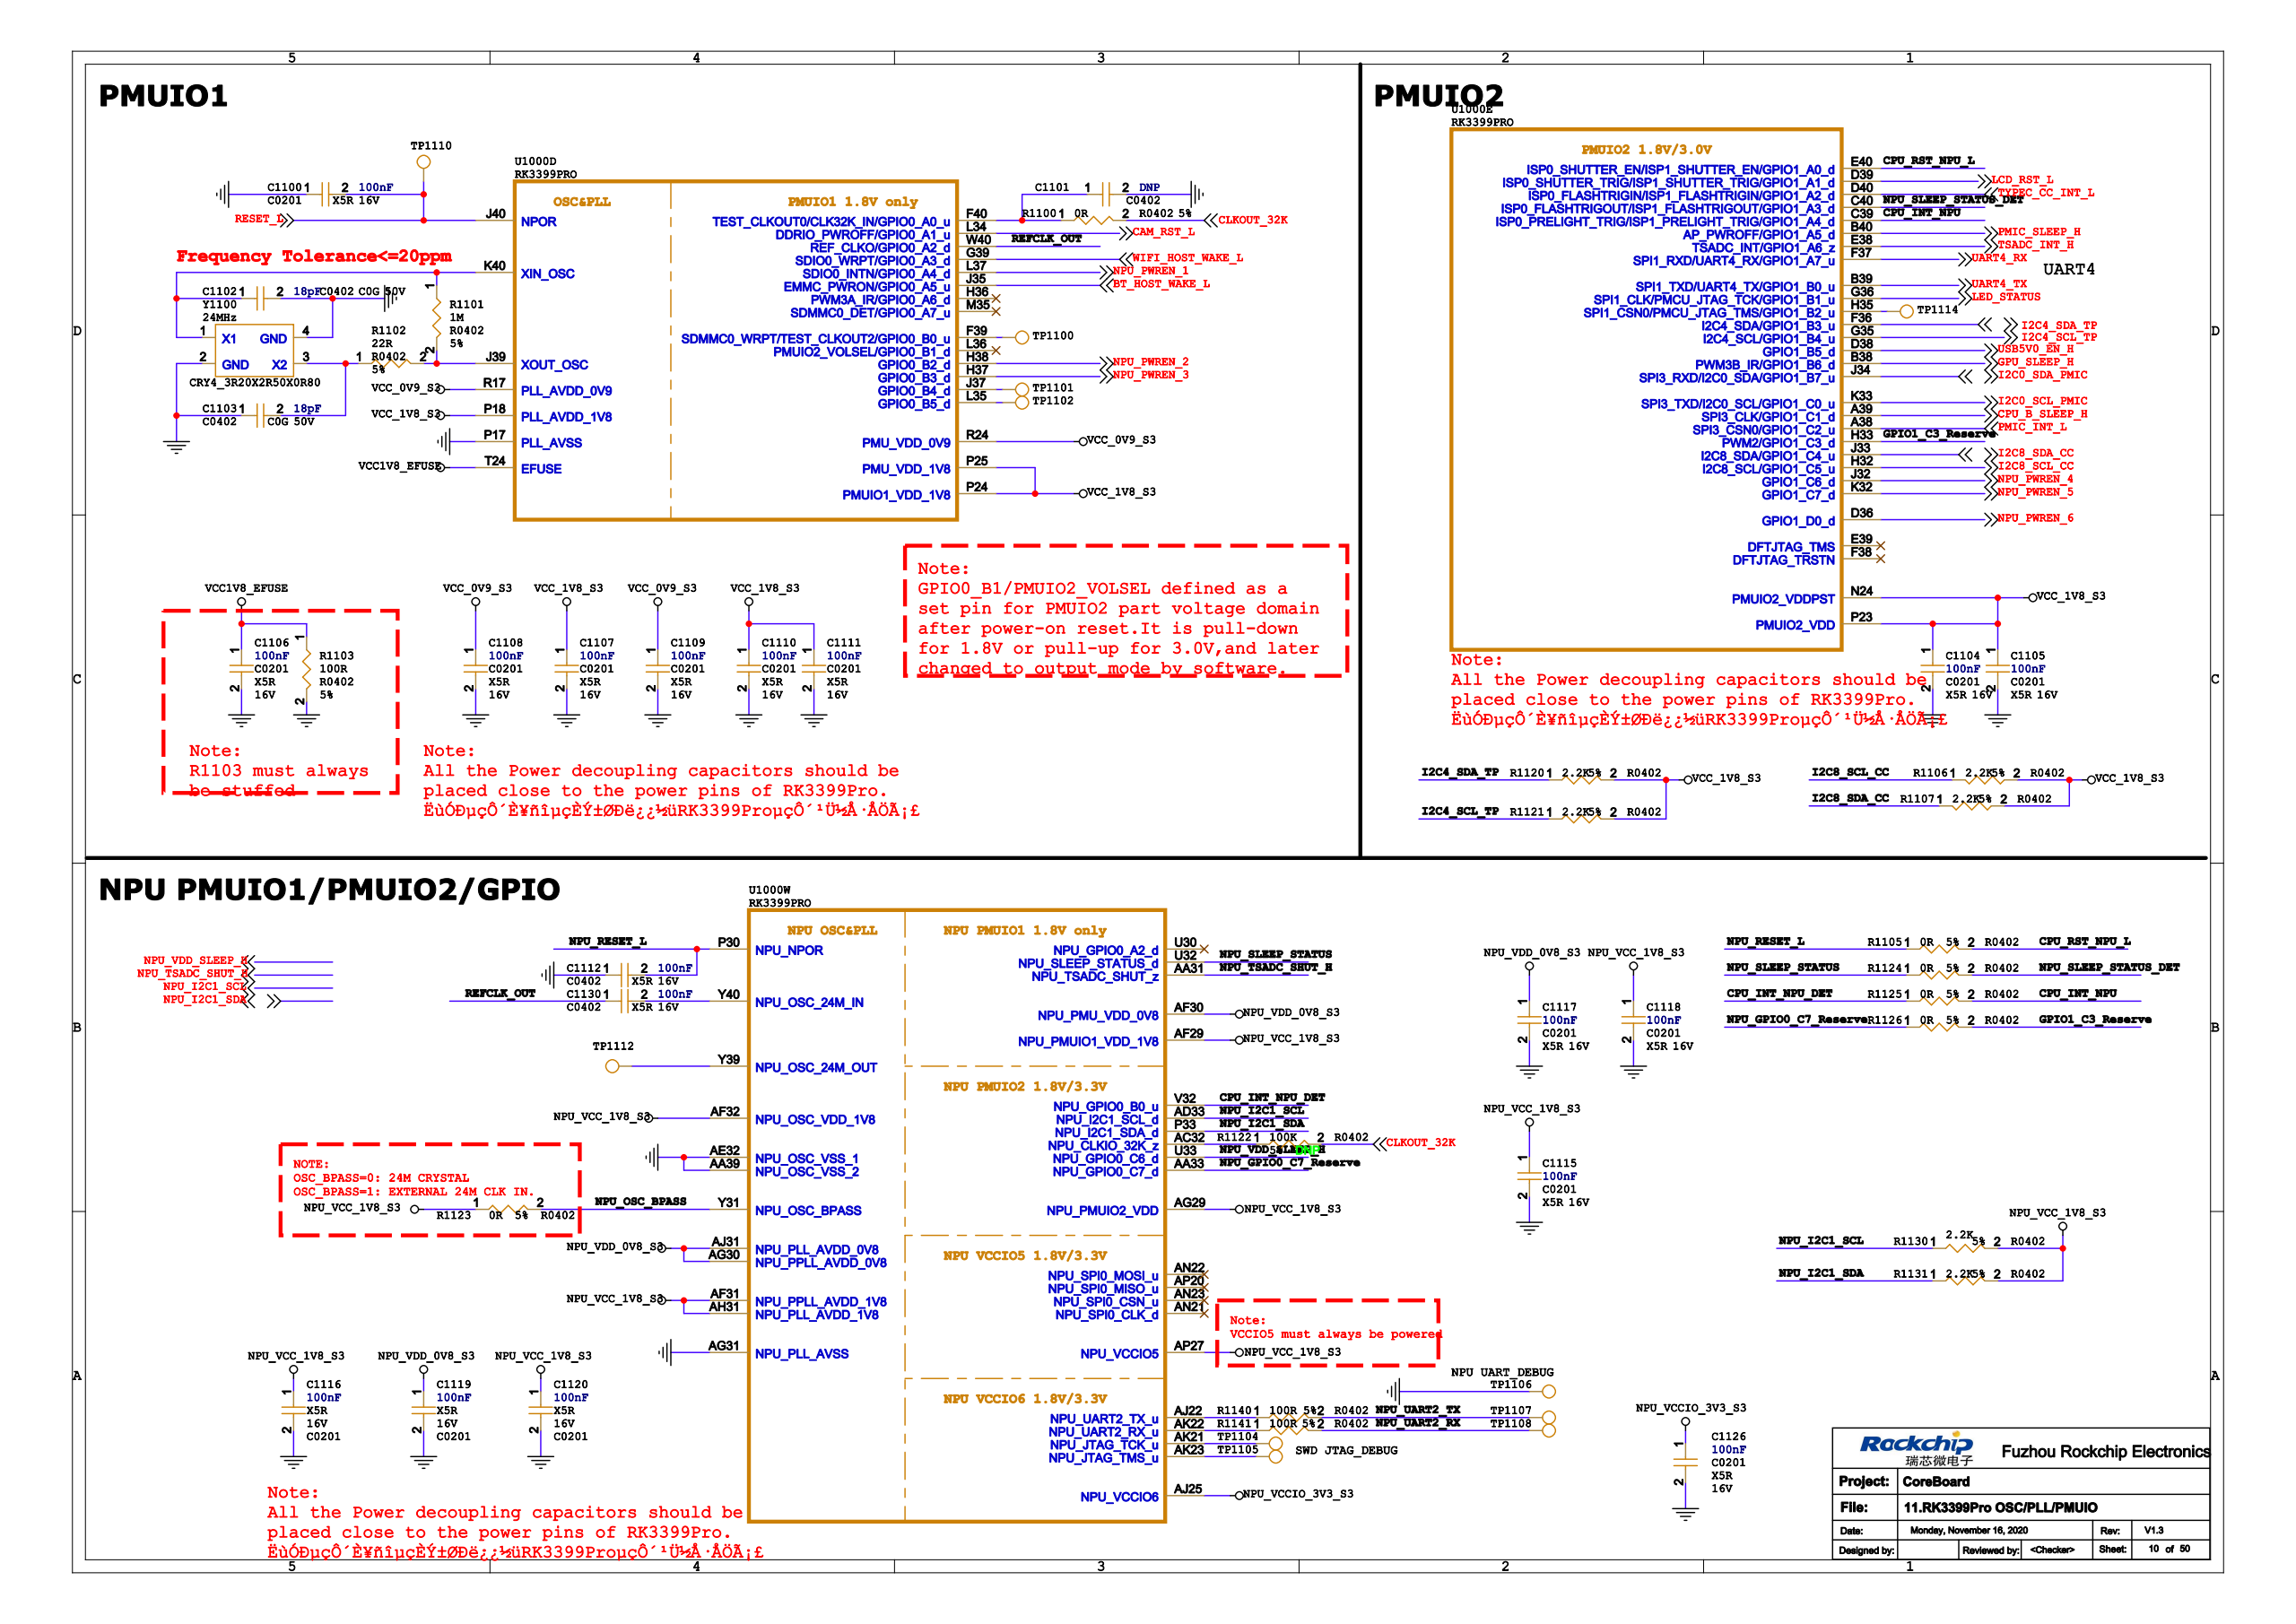Circuit board | Cadence Allegro | 749 parts | 717 nets | one sheet of the schematic
Parts on this sheet (reference | value | footprint):
C1100 | 100nF | C0201
C1101 | DNP | C0402
C1103 | 18pF | C0402
C1104 | 100nF | C0201
C1105 | 100nF | C0201
C1106 | 100nF | C0201
C1107 | 100nF | C0201
C1108 | 100nF | C0201
C1109 | 100nF | C0201
C1110 | 100nF | C0201
C1111 | 100nF | C0201
C1112 | 100nF | C0402
C1115 | 100nF | C0201
C1116 | 100nF | C0201
C1117 | 100nF | C0201
C1118 | 100nF | C0201
C1119 | 100nF | C0201
C1120 | 100nF | C0201
C1126 | 100nF | C0201
C1130 | 100nF | C0402
R1101 | 1M | R0402
R1102 | 22R | R0402
R1103 | 100R | R0402
R1122 | 100K | R0402
R1123 | 0R | R0402
R1130 | 2.2K | R0402
TP1100 | TP_0.5 | TP_10
TP1101 | TP_0.5 | TP_10
TP1102 | TP_0.5 | TP_10
TP1104 | TP_0.7 | TP_0R70
TP1105 | TP_0.7 | TP_0R70
TP1106 | TP_0.7 | TP_0R70
TP1107 | TP_0.7 | TP_0R70
TP1108 | TP_0.7 | TP_0R70
TP1110 | TP_0.7 | TP_0R70
TP1112 | TP_0.7 | TP_0R70
TP1114 | TP_0.5 | TP_10
U1000 | RK3399PRO | BGA1372_27R00X27R00X2R19
Y1100 | 24MHz | CRY4_3R20X2R50X0R80
Nets of these parts (net: part-pin ...):
GND: C1100-1 C1101-2 C1103-1 C1104-2 C1105-2 C1106-2 C1107-2 C1108-2 C1109-2 C1110-2 C1111-2 C1112-1 C1115-2 C1116-2 C1117-2 C1118-2 C1119-2 C1120-2 C1126-2 R1103-2 TP1106-1 Y1100-2 Y1100-4 U1000-AA39 U1000-AE32 U1000-AG31 U1000-P17
NPU_VCCIO_3V3_S3: C1126-1 U1000-AJ25
RESET_L: C1100-2 TP1110-1 U1000-J40
CLKOUT_32K: R1122-2
I2C4_SCL_TP: U1000-G35
I2C4_SDA_TP: U1000-F36
USB5V0_EN_H: U1000-D38
CAM_RST_L: U1000-L34
BT_HOST_WAKE_L: U1000-J35
LED_STATUS: U1000-G36
LCD_RST_L: U1000-D39
UART4_RX: U1000-F37
UART4_TX: U1000-B39
WIFI_HOST_WAKE_L: U1000-G39
TYPEC_CC_INT_L: U1000-D40
I2C8_SCL_CC: U1000-H32
I2C8_SDA_CC: U1000-J33
N18342843: TP1100-1 U1000-F39
N18342837: TP1101-1 U1000-J37
N18342840: TP1102-1 U1000-L35
N18342834: TP1114-1 U1000-H35
N78333897: C1101-1 U1000-F40
N82529146: R1101-1 Y1100-1 U1000-K40
N82529152: C1103-2 R1102-1 Y1100-3
NPU_VDD_0V8_S3: C1117-1 C1119-1 U1000-AF30 U1000-AG30 U1000-AJ31
NPU_VCC_1V8_S3: C1115-1 C1116-1 C1118-1 C1120-1 R1123-1 R1130-2 U1000-AF29 U1000-AF31 U1000-AF32 U1000-AG29 U1000-AH31 U1000-AP27
NPU_TSADC_SHUT_H: U1000-AA31
TSADC_INT_H: U1000-E38
N82547912: R1122-1 U1000-AC32
VCC_1V8_S3: C1104-1 C1105-1 C1107-1 C1110-1 C1111-1 U1000-N24 U1000-P18 U1000-P23 U1000-P24 U1000-P25
VCC_0V9_S3: C1108-1 C1109-1 U1000-R17 U1000-R24
VCC1V8_EFUSE: C1106-1 R1103-1 U1000-T24
NPU_PWREN_2: U1000-H38
NPU_PWREN_3: U1000-H37
REFCLK_OUT: C1130-1 U1000-W40
NPU_PWREN_1: U1000-L37
N82529148: R1101-2 R1102-2 U1000-J39
PMIC_SLEEP_H: U1000-B40
NPU_SLEEP_STATUS_DET: U1000-C40
CPU_INT_NPU: U1000-C39
CPU_RST_NPU_L: U1000-E40
GPU_SLEEP_H: U1000-B38
CPU_B_SLEEP_H: U1000-A39
PMIC_INT_L: U1000-A38
I2C0_SDA_PMIC: U1000-J34
I2C0_SCL_PMIC: U1000-K33
NPU_PWREN_4: U1000-J32
NPU_PWREN_5: U1000-K32
NPU_PWREN_6: U1000-D36
NPU_I2C1_SCL: R1130-1 U1000-AD33
NPU_I2C1_SDA: U1000-P33
N82548154: TP1104-1 U1000-AK21
N82548156: TP1105-1 U1000-AK23
CPU_INT_NPU_DET: U1000-V32
NPU_VDD_SLEEP_H: U1000-U33
NPU_RESET_L: C1112-2 U1000-P30
N82548939: C1130-2 U1000-Y40
N82548948: TP1112-1 U1000-Y39
NPU_OSC_BPASS: R1123-2 U1000-Y31
NPU_SLEEP_STATUS: U1000-U32
NPU_UART2_TX: TP1107-1
NPU_UART2_RX: TP1108-1